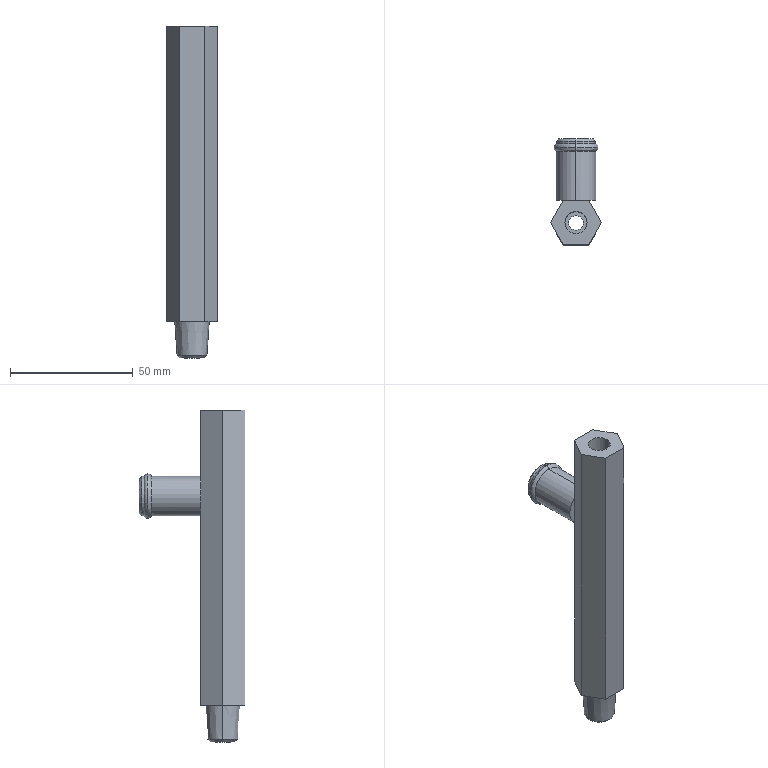Part | SolidWorks | features BaseBody 1 | 1 solid | 42 faces | box 20.785 x 43 x 135 mm | volume 30981 mm3 | plane 18 | cylinder 14 | cone 6 | spline 4 | commonest cylinder face diameters 9 x6 16 x4 6 x2 18 x2
STEP:
#1=CARTESIAN_POINT('',(0.,30.414,76.));
#2=VERTEX_POINT('',#1);
#3=CARTESIAN_POINT('',(0.,30.414,94.));
#4=VERTEX_POINT('',#3);
#5=CARTESIAN_POINT('',(0.,30.414,85.));
#6=DIRECTION('',(0.,-1.,0.));
#7=DIRECTION('',(0.,0.,-1.));
#8=AXIS2_PLACEMENT_3D('',#5,#6,#7);
#9=CIRCLE('',#8,9.);
#10=EDGE_CURVE('',#2,#4,#9,.T.);
#11=ORIENTED_EDGE('',*,*,#10,.T.);
#12=CARTESIAN_POINT('',(0.,29.,93.));
#13=VERTEX_POINT('',#12);
#14=CARTESIAN_POINT('',(0.,30.414,92.5));
#15=DIRECTION('',(1.,0.,0.));
#16=DIRECTION('',(0.,0.,1.));
#17=AXIS2_PLACEMENT_3D('',#14,#15,#16);
#18=CIRCLE('',#17,1.5);
#19=EDGE_CURVE('',#4,#13,#18,.T.);
#20=ORIENTED_EDGE('',*,*,#19,.T.);
#21=CARTESIAN_POINT('',(0.,29.,77.));
#22=VERTEX_POINT('',#21);
#23=CARTESIAN_POINT('',(0.,29.,85.));
#24=DIRECTION('',(0.,-1.,0.));
#25=DIRECTION('',(0.,0.,-1.));
#26=AXIS2_PLACEMENT_3D('',#23,#24,#25);
#27=CIRCLE('',#26,8.);
#28=EDGE_CURVE('',#22,#13,#27,.T.);
#29=ORIENTED_EDGE('',*,*,#28,.F.);
#30=CARTESIAN_POINT('',(0.,30.414,77.5));
#31=DIRECTION('',(-1.,0.,0.));
#32=DIRECTION('',(0.,0.,-1.));
#33=AXIS2_PLACEMENT_3D('',#30,#31,#32);
#34=CIRCLE('',#33,1.5);
#35=EDGE_CURVE('',#2,#22,#34,.T.);
#36=ORIENTED_EDGE('',*,*,#35,.F.);
#37=EDGE_LOOP('',(#11,#20,#29,#36));
#38=FACE_OUTER_BOUND('',#37,.T.);
#39=CARTESIAN_POINT('',(0.,30.414,94.));
#40=CARTESIAN_POINT('',(18.,30.414,94.));
#41=CARTESIAN_POINT('',(18.,30.414,76.));
#42=CARTESIAN_POINT('',(0.,30.414,76.));
#43=CARTESIAN_POINT('',(0.,29.756,94.));
#44=CARTESIAN_POINT('',(18.,29.756,94.));
#45=CARTESIAN_POINT('',(18.,29.756,76.));
#46=CARTESIAN_POINT('',(0.,29.756,76.));
#47=CARTESIAN_POINT('',(0.,29.219,93.62));
#48=CARTESIAN_POINT('',(17.24,29.219,93.62));
#49=CARTESIAN_POINT('',(17.24,29.219,76.38));
#50=CARTESIAN_POINT('',(0.,29.219,76.38));
#51=CARTESIAN_POINT('',(0.,29.,93.));
#52=CARTESIAN_POINT('',(16.,29.,93.));
#53=CARTESIAN_POINT('',(16.,29.,77.));
#54=CARTESIAN_POINT('',(0.,29.,77.));
#55=(BOUNDED_SURFACE()B_SPLINE_SURFACE(3,3,((#39,#40,#41,#42),(#43,#44,#45,#46),(#47,#48,#49,#50),(#51,#52,#53,#54)),.UNSPECIFIED.,.F.,.F.,.T.)B_SPLINE_SURFACE_WITH_KNOTS((4,4),(4,4),(0.,1.),(0.,1.),.UNSPECIFIED.)GEOMETRIC_REPRESENTATION_ITEM()RATIONAL_B_SPLINE_SURFACE(((1.,0.3333,0.3333,1.),(0.8777,0.2926,0.2926,0.8777),(0.8777,0.2926,0.2926,0.8777),(1.,0.3333,0.3333,1.)))REPRESENTATION_ITEM('')SURFACE());
#56=ADVANCED_FACE('',(#38),#55,.T.);
#57=CARTESIAN_POINT('',(0.,30.586,94.));
#58=VERTEX_POINT('',#57);
#59=CARTESIAN_POINT('',(0.,30.586,76.));
#60=VERTEX_POINT('',#59);
#61=CARTESIAN_POINT('',(0.,30.586,85.));
#62=DIRECTION('',(0.,-1.,0.));
#63=DIRECTION('',(0.,0.,1.));
#64=AXIS2_PLACEMENT_3D('',#61,#62,#63);
#65=CIRCLE('',#64,9.);
#66=EDGE_CURVE('',#58,#60,#65,.T.);
#67=ORIENTED_EDGE('',*,*,#66,.F.);
#68=CARTESIAN_POINT('',(0.,32.,93.));
#69=VERTEX_POINT('',#68);
#70=CARTESIAN_POINT('',(0.,30.586,92.5));
#71=DIRECTION('',(-1.,0.,0.));
#72=DIRECTION('',(0.,0.,1.));
#73=AXIS2_PLACEMENT_3D('',#70,#71,#72);
#74=CIRCLE('',#73,1.5);
#75=EDGE_CURVE('',#58,#69,#74,.T.);
#76=ORIENTED_EDGE('',*,*,#75,.T.);
#77=CARTESIAN_POINT('',(0.,32.,77.));
#78=VERTEX_POINT('',#77);
#79=CARTESIAN_POINT('',(0.,32.,85.));
#80=DIRECTION('',(0.,-1.,0.));
#81=DIRECTION('',(0.,0.,-1.));
#82=AXIS2_PLACEMENT_3D('',#79,#80,#81);
#83=CIRCLE('',#82,8.);
#84=EDGE_CURVE('',#69,#78,#83,.T.);
#85=ORIENTED_EDGE('',*,*,#84,.T.);
#86=CARTESIAN_POINT('',(0.,30.586,77.5));
#87=DIRECTION('',(1.,0.,0.));
#88=DIRECTION('',(0.,0.,-1.));
#89=AXIS2_PLACEMENT_3D('',#86,#87,#88);
#90=CIRCLE('',#89,1.5);
#91=EDGE_CURVE('',#60,#78,#90,.T.);
#92=ORIENTED_EDGE('',*,*,#91,.F.);
#93=EDGE_LOOP('',(#67,#76,#85,#92));
#94=FACE_OUTER_BOUND('',#93,.T.);
#95=CARTESIAN_POINT('',(0.,30.586,94.));
#96=CARTESIAN_POINT('',(-18.,30.586,94.));
#97=CARTESIAN_POINT('',(-18.,30.586,76.));
#98=CARTESIAN_POINT('',(0.,30.586,76.));
#99=CARTESIAN_POINT('',(0.,31.244,94.));
#100=CARTESIAN_POINT('',(-18.,31.244,94.));
#101=CARTESIAN_POINT('',(-18.,31.244,76.));
#102=CARTESIAN_POINT('',(0.,31.244,76.));
#103=CARTESIAN_POINT('',(0.,31.781,93.62));
#104=CARTESIAN_POINT('',(-17.24,31.781,93.62));
#105=CARTESIAN_POINT('',(-17.24,31.781,76.38));
#106=CARTESIAN_POINT('',(0.,31.781,76.38));
#107=CARTESIAN_POINT('',(0.,32.,93.));
#108=CARTESIAN_POINT('',(-16.,32.,93.));
#109=CARTESIAN_POINT('',(-16.,32.,77.));
#110=CARTESIAN_POINT('',(0.,32.,77.));
#111=(BOUNDED_SURFACE()B_SPLINE_SURFACE(3,3,((#95,#96,#97,#98),(#99,#100,#101,#102),(#103,#104,#105,#106),(#107,#108,#109,#110)),.UNSPECIFIED.,.F.,.F.,.F.)B_SPLINE_SURFACE_WITH_KNOTS((4,4),(4,4),(0.,1.),(0.,1.),.UNSPECIFIED.)GEOMETRIC_REPRESENTATION_ITEM()RATIONAL_B_SPLINE_SURFACE(((1.,0.3333,0.3333,1.),(0.8777,0.2926,0.2926,0.8777),(0.8777,0.2926,0.2926,0.8777),(1.,0.3333,0.3333,1.)))REPRESENTATION_ITEM('')SURFACE());
#112=ADVANCED_FACE('',(#94),#111,.T.);
#113=CARTESIAN_POINT('',(4.5,0.,120.));
#114=VERTEX_POINT('',#113);
#115=CARTESIAN_POINT('',(-4.5,0.,120.));
#116=VERTEX_POINT('',#115);
#117=CARTESIAN_POINT('',(0.,0.,120.));
#118=DIRECTION('',(0.,0.,-1.));
#119=DIRECTION('',(-1.,0.,0.));
#120=AXIS2_PLACEMENT_3D('',#117,#118,#119);
#121=CIRCLE('',#120,4.5);
#122=EDGE_CURVE('',#114,#116,#121,.T.);
#123=ORIENTED_EDGE('',*,*,#122,.F.);
#124=CARTESIAN_POINT('',(4.5,0.,0.));
#125=VERTEX_POINT('',#124);
#126=CARTESIAN_POINT('',(4.5,0.,120.));
#127=DIRECTION('',(0.,0.,-1.));
#128=VECTOR('',#127,1000.);
#129=LINE('',#126,#128);
#130=EDGE_CURVE('',#114,#125,#129,.T.);
#131=ORIENTED_EDGE('',*,*,#130,.T.);
#132=CARTESIAN_POINT('',(-4.5,0.,0.));
#133=VERTEX_POINT('',#132);
#134=CARTESIAN_POINT('',(0.,0.,0.));
#135=DIRECTION('',(0.,0.,1.));
#136=DIRECTION('',(-1.,0.,0.));
#137=AXIS2_PLACEMENT_3D('',#134,#135,#136);
#138=CIRCLE('',#137,4.5);
#139=EDGE_CURVE('',#133,#125,#138,.T.);
#140=ORIENTED_EDGE('',*,*,#139,.F.);
#141=CARTESIAN_POINT('',(-4.5,0.,120.));
#142=DIRECTION('',(0.,0.,-1.));
#143=VECTOR('',#142,1000.);
#144=LINE('',#141,#143);
#145=EDGE_CURVE('',#116,#133,#144,.T.);
#146=ORIENTED_EDGE('',*,*,#145,.F.);
#147=EDGE_LOOP('',(#123,#131,#140,#146));
#148=FACE_OUTER_BOUND('',#147,.T.);
#149=CARTESIAN_POINT('',(0.,0.,120.));
#150=DIRECTION('',(0.,0.,-1.));
#151=DIRECTION('',(-1.,0.,0.));
#152=AXIS2_PLACEMENT_3D('',#149,#150,#151);
#153=CYLINDRICAL_SURFACE('',#152,4.5);
#154=ADVANCED_FACE('',(#148),#153,.F.);
#155=CARTESIAN_POINT('',(-4.031,2.,83.));
#156=VERTEX_POINT('',#155);
#157=CARTESIAN_POINT('',(0.,4.5,80.5));
#158=VERTEX_POINT('',#157);
#159=CARTESIAN_POINT('',(-4.031,2.,83.));
#160=CARTESIAN_POINT('',(-3.25,3.574,81.426));
#161=CARTESIAN_POINT('',(-1.757,4.5,80.5));
#162=CARTESIAN_POINT('',(0.,4.5,80.5));
#163=(BOUNDED_CURVE()B_SPLINE_CURVE(3,(#159,#160,#161,#162),.UNSPECIFIED.,.F.,.T.)B_SPLINE_CURVE_WITH_KNOTS((4,4),(5.173,6.283),.UNSPECIFIED.)CURVE()GEOMETRIC_REPRESENTATION_ITEM()RATIONAL_B_SPLINE_CURVE((1.,0.8999,0.8999,1.))REPRESENTATION_ITEM(''));
#164=EDGE_CURVE('',#156,#158,#163,.T.);
#165=ORIENTED_EDGE('',*,*,#164,.T.);
#166=CARTESIAN_POINT('',(0.,29.,80.5));
#167=VERTEX_POINT('',#166);
#168=CARTESIAN_POINT('',(0.,2.,80.5));
#169=DIRECTION('',(0.,1.,0.));
#170=VECTOR('',#169,1000.);
#171=LINE('',#168,#170);
#172=EDGE_CURVE('',#158,#167,#171,.T.);
#173=ORIENTED_EDGE('',*,*,#172,.T.);
#174=CARTESIAN_POINT('',(0.,29.,89.5));
#175=VERTEX_POINT('',#174);
#176=CARTESIAN_POINT('',(0.,29.,85.));
#177=DIRECTION('',(0.,-1.,0.));
#178=DIRECTION('',(0.,0.,1.));
#179=AXIS2_PLACEMENT_3D('',#176,#177,#178);
#180=CIRCLE('',#179,4.5);
#181=EDGE_CURVE('',#175,#167,#180,.T.);
#182=ORIENTED_EDGE('',*,*,#181,.F.);
#183=CARTESIAN_POINT('',(0.,4.5,89.5));
#184=VERTEX_POINT('',#183);
#185=CARTESIAN_POINT('',(0.,2.,89.5));
#186=DIRECTION('',(0.,1.,0.));
#187=VECTOR('',#186,1000.);
#188=LINE('',#185,#187);
#189=EDGE_CURVE('',#184,#175,#188,.T.);
#190=ORIENTED_EDGE('',*,*,#189,.F.);
#191=CARTESIAN_POINT('',(-4.031,2.,87.));
#192=VERTEX_POINT('',#191);
#193=CARTESIAN_POINT('',(0.,4.5,89.5));
#194=CARTESIAN_POINT('',(-1.757,4.5,89.5));
#195=CARTESIAN_POINT('',(-3.25,3.574,88.574));
#196=CARTESIAN_POINT('',(-4.031,2.,87.));
#197=(BOUNDED_CURVE()B_SPLINE_CURVE(3,(#193,#194,#195,#196),.UNSPECIFIED.,.F.,.F.)B_SPLINE_CURVE_WITH_KNOTS((4,4),(0.,1.11),.UNSPECIFIED.)CURVE()GEOMETRIC_REPRESENTATION_ITEM()RATIONAL_B_SPLINE_CURVE((1.,0.8999,0.8999,1.))REPRESENTATION_ITEM(''));
#198=EDGE_CURVE('',#184,#192,#197,.T.);
#199=ORIENTED_EDGE('',*,*,#198,.T.);
#200=CARTESIAN_POINT('',(0.,2.,85.));
#201=DIRECTION('',(0.,1.,0.));
#202=DIRECTION('',(0.,0.,1.));
#203=AXIS2_PLACEMENT_3D('',#200,#201,#202);
#204=CIRCLE('',#203,4.5);
#205=EDGE_CURVE('',#156,#192,#204,.T.);
#206=ORIENTED_EDGE('',*,*,#205,.F.);
#207=EDGE_LOOP('',(#165,#173,#182,#190,#199,#206));
#208=FACE_OUTER_BOUND('',#207,.T.);
#209=CARTESIAN_POINT('',(0.,2.,85.));
#210=DIRECTION('',(0.,1.,0.));
#211=DIRECTION('',(0.,0.,1.));
#212=AXIS2_PLACEMENT_3D('',#209,#210,#211);
#213=CYLINDRICAL_SURFACE('',#212,4.5);
#214=ADVANCED_FACE('',(#208),#213,.F.);
#215=CARTESIAN_POINT('',(3.,0.,0.));
#216=VERTEX_POINT('',#215);
#217=CARTESIAN_POINT('',(-3.,0.,0.));
#218=VERTEX_POINT('',#217);
#219=CARTESIAN_POINT('',(0.,0.,0.));
#220=DIRECTION('',(0.,0.,-1.));
#221=DIRECTION('',(-1.,0.,0.));
#222=AXIS2_PLACEMENT_3D('',#219,#220,#221);
#223=CIRCLE('',#222,3.);
#224=EDGE_CURVE('',#216,#218,#223,.T.);
#225=ORIENTED_EDGE('',*,*,#224,.F.);
#226=CARTESIAN_POINT('',(3.,0.,-15.));
#227=VERTEX_POINT('',#226);
#228=CARTESIAN_POINT('',(3.,0.,0.));
#229=DIRECTION('',(0.,0.,-1.));
#230=VECTOR('',#229,1000.);
#231=LINE('',#228,#230);
#232=EDGE_CURVE('',#216,#227,#231,.T.);
#233=ORIENTED_EDGE('',*,*,#232,.T.);
#234=CARTESIAN_POINT('',(-3.,0.,-15.));
#235=VERTEX_POINT('',#234);
#236=CARTESIAN_POINT('',(0.,0.,-15.));
#237=DIRECTION('',(0.,0.,1.));
#238=DIRECTION('',(-1.,0.,0.));
#239=AXIS2_PLACEMENT_3D('',#236,#237,#238);
#240=CIRCLE('',#239,3.);
#241=EDGE_CURVE('',#235,#227,#240,.T.);
#242=ORIENTED_EDGE('',*,*,#241,.F.);
#243=CARTESIAN_POINT('',(-3.,0.,0.));
#244=DIRECTION('',(0.,0.,-1.));
#245=VECTOR('',#244,1000.);
#246=LINE('',#243,#245);
#247=EDGE_CURVE('',#218,#235,#246,.T.);
#248=ORIENTED_EDGE('',*,*,#247,.F.);
#249=EDGE_LOOP('',(#225,#233,#242,#248));
#250=FACE_OUTER_BOUND('',#249,.T.);
#251=CARTESIAN_POINT('',(0.,0.,0.));
#252=DIRECTION('',(0.,0.,-1.));
#253=DIRECTION('',(-1.,0.,0.));
#254=AXIS2_PLACEMENT_3D('',#251,#252,#253);
#255=CYLINDRICAL_SURFACE('',#254,3.);
#256=ADVANCED_FACE('',(#250),#255,.F.);
#257=ORIENTED_EDGE('',*,*,#28,.T.);
#258=CARTESIAN_POINT('',(0.,9.,93.));
#259=VERTEX_POINT('',#258);
#260=CARTESIAN_POINT('',(0.,29.,93.));
#261=DIRECTION('',(0.,-1.,0.));
#262=VECTOR('',#261,1000.);
#263=LINE('',#260,#262);
#264=EDGE_CURVE('',#13,#259,#263,.T.);
#265=ORIENTED_EDGE('',*,*,#264,.T.);
#266=CARTESIAN_POINT('',(5.196,9.,91.083));
#267=VERTEX_POINT('',#266);
#268=CARTESIAN_POINT('',(0.,9.,85.));
#269=DIRECTION('',(0.,-1.,0.));
#270=DIRECTION('',(0.,0.,-1.));
#271=AXIS2_PLACEMENT_3D('',#268,#269,#270);
#272=CIRCLE('',#271,8.);
#273=EDGE_CURVE('',#267,#259,#272,.T.);
#274=ORIENTED_EDGE('',*,*,#273,.F.);
#275=CARTESIAN_POINT('',(5.196,9.,78.917));
#276=VERTEX_POINT('',#275);
#277=CARTESIAN_POINT('',(0.,9.,85.));
#278=DIRECTION('',(0.,1.,0.));
#279=DIRECTION('',(0.,0.,-1.));
#280=AXIS2_PLACEMENT_3D('',#277,#278,#279);
#281=CIRCLE('',#280,8.);
#282=EDGE_CURVE('',#267,#276,#281,.T.);
#283=ORIENTED_EDGE('',*,*,#282,.T.);
#284=CARTESIAN_POINT('',(0.,9.,77.));
#285=VERTEX_POINT('',#284);
#286=CARTESIAN_POINT('',(0.,9.,85.));
#287=DIRECTION('',(0.,-1.,0.));
#288=DIRECTION('',(0.,0.,-1.));
#289=AXIS2_PLACEMENT_3D('',#286,#287,#288);
#290=CIRCLE('',#289,8.);
#291=EDGE_CURVE('',#285,#276,#290,.T.);
#292=ORIENTED_EDGE('',*,*,#291,.F.);
#293=CARTESIAN_POINT('',(0.,29.,77.));
#294=DIRECTION('',(0.,-1.,0.));
#295=VECTOR('',#294,1000.);
#296=LINE('',#293,#295);
#297=EDGE_CURVE('',#22,#285,#296,.T.);
#298=ORIENTED_EDGE('',*,*,#297,.F.);
#299=EDGE_LOOP('',(#257,#265,#274,#283,#292,#298));
#300=FACE_OUTER_BOUND('',#299,.T.);
#301=CARTESIAN_POINT('',(0.,29.,85.));
#302=DIRECTION('',(0.,-1.,0.));
#303=DIRECTION('',(0.,0.,-1.));
#304=AXIS2_PLACEMENT_3D('',#301,#302,#303);
#305=CYLINDRICAL_SURFACE('',#304,8.);
#306=ADVANCED_FACE('',(#300),#305,.T.);
#307=CARTESIAN_POINT('',(6.071,0.,-13.929));
#308=VERTEX_POINT('',#307);
#309=CARTESIAN_POINT('',(-6.071,0.,-13.929));
#310=VERTEX_POINT('',#309);
#311=CARTESIAN_POINT('',(0.,0.,-13.929));
#312=DIRECTION('',(0.,0.,1.));
#313=DIRECTION('',(1.,0.,0.));
#314=AXIS2_PLACEMENT_3D('',#311,#312,#313);
#315=CIRCLE('',#314,6.071);
#316=EDGE_CURVE('',#308,#310,#315,.T.);
#317=ORIENTED_EDGE('',*,*,#316,.T.);
#318=CARTESIAN_POINT('',(-7.,0.,0.));
#319=VERTEX_POINT('',#318);
#320=CARTESIAN_POINT('',(-7.,0.,0.));
#321=DIRECTION('',(-0.06652,0.,0.9978));
#322=VECTOR('',#321,1000.);
#323=LINE('',#320,#322);
#324=EDGE_CURVE('',#310,#319,#323,.T.);
#325=ORIENTED_EDGE('',*,*,#324,.T.);
#326=CARTESIAN_POINT('',(7.,0.,0.));
#327=VERTEX_POINT('',#326);
#328=CARTESIAN_POINT('',(0.,0.,0.));
#329=DIRECTION('',(0.,0.,-1.));
#330=DIRECTION('',(1.,0.,0.));
#331=AXIS2_PLACEMENT_3D('',#328,#329,#330);
#332=CIRCLE('',#331,7.);
#333=EDGE_CURVE('',#319,#327,#332,.T.);
#334=ORIENTED_EDGE('',*,*,#333,.T.);
#335=CARTESIAN_POINT('',(7.,0.,0.));
#336=DIRECTION('',(0.06652,0.,0.9978));
#337=VECTOR('',#336,1000.);
#338=LINE('',#335,#337);
#339=EDGE_CURVE('',#308,#327,#338,.T.);
#340=ORIENTED_EDGE('',*,*,#339,.F.);
#341=EDGE_LOOP('',(#317,#325,#334,#340));
#342=FACE_OUTER_BOUND('',#341,.T.);
#343=CARTESIAN_POINT('',(0.,0.,0.));
#344=DIRECTION('',(0.,0.,1.));
#345=DIRECTION('',(1.,0.,0.));
#346=AXIS2_PLACEMENT_3D('',#343,#344,#345);
#347=CONICAL_SURFACE('',#346,7.,0.06657);
#348=ADVANCED_FACE('',(#342),#347,.T.);
#349=CARTESIAN_POINT('',(5.,0.,-15.));
#350=VERTEX_POINT('',#349);
#351=CARTESIAN_POINT('',(-5.,0.,-15.));
#352=VERTEX_POINT('',#351);
#353=CARTESIAN_POINT('',(0.,0.,-15.));
#354=DIRECTION('',(0.,0.,1.));
#355=DIRECTION('',(1.,0.,0.));
#356=AXIS2_PLACEMENT_3D('',#353,#354,#355);
#357=CIRCLE('',#356,5.);
#358=EDGE_CURVE('',#350,#352,#357,.T.);
#359=ORIENTED_EDGE('',*,*,#358,.T.);
#360=CARTESIAN_POINT('',(-6.071,0.,-13.929));
#361=DIRECTION('',(-0.7071,0.,0.7071));
#362=VECTOR('',#361,1000.);
#363=LINE('',#360,#362);
#364=EDGE_CURVE('',#352,#310,#363,.T.);
#365=ORIENTED_EDGE('',*,*,#364,.T.);
#366=ORIENTED_EDGE('',*,*,#316,.F.);
#367=CARTESIAN_POINT('',(6.071,0.,-13.929));
#368=DIRECTION('',(0.7071,0.,0.7071));
#369=VECTOR('',#368,1000.);
#370=LINE('',#367,#369);
#371=EDGE_CURVE('',#350,#308,#370,.T.);
#372=ORIENTED_EDGE('',*,*,#371,.F.);
#373=EDGE_LOOP('',(#359,#365,#366,#372));
#374=FACE_OUTER_BOUND('',#373,.T.);
#375=CARTESIAN_POINT('',(0.,0.,-13.929));
#376=DIRECTION('',(0.,0.,1.));
#377=DIRECTION('',(1.,0.,0.));
#378=AXIS2_PLACEMENT_3D('',#375,#376,#377);
#379=CONICAL_SURFACE('',#378,6.071,0.7854);
#380=ADVANCED_FACE('',(#374),#379,.T.);
#381=ORIENTED_EDGE('',*,*,#10,.F.);
#382=CARTESIAN_POINT('',(0.,30.414,76.));
#383=DIRECTION('',(0.,1.,0.));
#384=VECTOR('',#383,1000.);
#385=LINE('',#382,#384);
#386=EDGE_CURVE('',#2,#60,#385,.T.);
#387=ORIENTED_EDGE('',*,*,#386,.T.);
#388=CARTESIAN_POINT('',(0.,30.586,85.));
#389=DIRECTION('',(0.,-1.,0.));
#390=DIRECTION('',(0.,0.,1.));
#391=AXIS2_PLACEMENT_3D('',#388,#389,#390);
#392=CIRCLE('',#391,9.);
#393=EDGE_CURVE('',#60,#58,#392,.T.);
#394=ORIENTED_EDGE('',*,*,#393,.T.);
#395=CARTESIAN_POINT('',(0.,30.414,94.));
#396=DIRECTION('',(0.,1.,0.));
#397=VECTOR('',#396,1000.);
#398=LINE('',#395,#397);
#399=EDGE_CURVE('',#4,#58,#398,.T.);
#400=ORIENTED_EDGE('',*,*,#399,.F.);
#401=EDGE_LOOP('',(#381,#387,#394,#400));
#402=FACE_OUTER_BOUND('',#401,.T.);
#403=CARTESIAN_POINT('',(0.,30.414,85.));
#404=DIRECTION('',(0.,1.,0.));
#405=DIRECTION('',(0.,0.,1.));
#406=AXIS2_PLACEMENT_3D('',#403,#404,#405);
#407=CYLINDRICAL_SURFACE('',#406,9.);
#408=ADVANCED_FACE('',(#402),#407,.T.);
#409=CARTESIAN_POINT('',(0.,33.,77.));
#410=VERTEX_POINT('',#409);
#411=CARTESIAN_POINT('',(0.,33.,93.));
#412=VERTEX_POINT('',#411);
#413=CARTESIAN_POINT('',(0.,33.,85.));
#414=DIRECTION('',(0.,-1.,0.));
#415=DIRECTION('',(0.,0.,-1.));
#416=AXIS2_PLACEMENT_3D('',#413,#414,#415);
#417=CIRCLE('',#416,8.);
#418=EDGE_CURVE('',#410,#412,#417,.T.);
#419=ORIENTED_EDGE('',*,*,#418,.T.);
#420=CARTESIAN_POINT('',(0.,33.,93.));
#421=DIRECTION('',(0.,-1.,0.));
#422=VECTOR('',#421,1000.);
#423=LINE('',#420,#422);
#424=EDGE_CURVE('',#412,#69,#423,.T.);
#425=ORIENTED_EDGE('',*,*,#424,.T.);
#426=CARTESIAN_POINT('',(0.,32.,85.));
#427=DIRECTION('',(0.,-1.,0.));
#428=DIRECTION('',(0.,0.,-1.));
#429=AXIS2_PLACEMENT_3D('',#426,#427,#428);
#430=CIRCLE('',#429,8.);
#431=EDGE_CURVE('',#78,#69,#430,.T.);
#432=ORIENTED_EDGE('',*,*,#431,.F.);
#433=CARTESIAN_POINT('',(0.,33.,77.));
#434=DIRECTION('',(0.,-1.,0.));
#435=VECTOR('',#434,1000.);
#436=LINE('',#433,#435);
#437=EDGE_CURVE('',#410,#78,#436,.T.);
#438=ORIENTED_EDGE('',*,*,#437,.F.);
#439=EDGE_LOOP('',(#419,#425,#432,#438));
#440=FACE_OUTER_BOUND('',#439,.T.);
#441=CARTESIAN_POINT('',(0.,33.,85.));
#442=DIRECTION('',(0.,-1.,0.));
#443=DIRECTION('',(0.,0.,-1.));
#444=AXIS2_PLACEMENT_3D('',#441,#442,#443);
#445=CYLINDRICAL_SURFACE('',#444,8.);
#446=ADVANCED_FACE('',(#440),#445,.T.);
#447=CARTESIAN_POINT('',(0.,34.,78.));
#448=VERTEX_POINT('',#447);
#449=CARTESIAN_POINT('',(0.,34.,92.));
#450=VERTEX_POINT('',#449);
#451=CARTESIAN_POINT('',(0.,34.,85.));
#452=DIRECTION('',(0.,-1.,0.));
#453=DIRECTION('',(0.,0.,-1.));
#454=AXIS2_PLACEMENT_3D('',#451,#452,#453);
#455=CIRCLE('',#454,7.);
#456=EDGE_CURVE('',#448,#450,#455,.T.);
#457=ORIENTED_EDGE('',*,*,#456,.T.);
#458=CARTESIAN_POINT('',(0.,33.,93.));
#459=DIRECTION('',(0.,-0.7071,0.7071));
#460=VECTOR('',#459,1000.);
#461=LINE('',#458,#460);
#462=EDGE_CURVE('',#450,#412,#461,.T.);
#463=ORIENTED_EDGE('',*,*,#462,.T.);
#464=ORIENTED_EDGE('',*,*,#418,.F.);
#465=CARTESIAN_POINT('',(0.,33.,77.));
#466=DIRECTION('',(0.,-0.7071,-0.7071));
#467=VECTOR('',#466,1000.);
#468=LINE('',#465,#467);
#469=EDGE_CURVE('',#448,#410,#468,.T.);
#470=ORIENTED_EDGE('',*,*,#469,.F.);
#471=EDGE_LOOP('',(#457,#463,#464,#470));
#472=FACE_OUTER_BOUND('',#471,.T.);
#473=CARTESIAN_POINT('',(0.,33.,85.));
#474=DIRECTION('',(0.,-1.,0.));
#475=DIRECTION('',(0.,0.,-1.));
#476=AXIS2_PLACEMENT_3D('',#473,#474,#475);
#477=CONICAL_SURFACE('',#476,8.,0.7854);
#478=ADVANCED_FACE('',(#472),#477,.T.);
#479=CARTESIAN_POINT('',(0.,34.,89.5));
#480=VERTEX_POINT('',#479);
#481=CARTESIAN_POINT('',(0.,34.,80.5));
#482=VERTEX_POINT('',#481);
#483=CARTESIAN_POINT('',(0.,34.,85.));
#484=DIRECTION('',(0.,-1.,0.));
#485=DIRECTION('',(0.,0.,-1.));
#486=AXIS2_PLACEMENT_3D('',#483,#484,#485);
#487=CIRCLE('',#486,4.5);
#488=EDGE_CURVE('',#480,#482,#487,.T.);
#489=ORIENTED_EDGE('',*,*,#488,.F.);
#490=CARTESIAN_POINT('',(0.,32.,89.5));
#491=VERTEX_POINT('',#490);
#492=CARTESIAN_POINT('',(0.,34.,89.5));
#493=DIRECTION('',(0.,-1.,0.));
#494=VECTOR('',#493,1000.);
#495=LINE('',#492,#494);
#496=EDGE_CURVE('',#480,#491,#495,.T.);
#497=ORIENTED_EDGE('',*,*,#496,.T.);
#498=CARTESIAN_POINT('',(0.,32.,80.5));
#499=VERTEX_POINT('',#498);
#500=CARTESIAN_POINT('',(0.,32.,85.));
#501=DIRECTION('',(0.,1.,0.));
#502=DIRECTION('',(0.,0.,-1.));
#503=AXIS2_PLACEMENT_3D('',#500,#501,#502);
#504=CIRCLE('',#503,4.5);
#505=EDGE_CURVE('',#499,#491,#504,.T.);
#506=ORIENTED_EDGE('',*,*,#505,.F.);
#507=CARTESIAN_POINT('',(0.,34.,80.5));
#508=DIRECTION('',(0.,-1.,0.));
#509=VECTOR('',#508,1000.);
#510=LINE('',#507,#509);
#511=EDGE_CURVE('',#482,#499,#510,.T.);
#512=ORIENTED_EDGE('',*,*,#511,.F.);
#513=EDGE_LOOP('',(#489,#497,#506,#512));
#514=FACE_OUTER_BOUND('',#513,.T.);
#515=CARTESIAN_POINT('',(0.,34.,85.));
#516=DIRECTION('',(0.,-1.,0.));
#517=DIRECTION('',(0.,0.,-1.));
#518=AXIS2_PLACEMENT_3D('',#515,#516,#517);
#519=CYLINDRICAL_SURFACE('',#518,4.5);
#520=ADVANCED_FACE('',(#514),#519,.F.);
#521=ORIENTED_EDGE('',*,*,#130,.F.);
#522=CARTESIAN_POINT('',(0.,0.,120.));
#523=DIRECTION('',(0.,0.,-1.));
#524=DIRECTION('',(-1.,0.,0.));
#525=AXIS2_PLACEMENT_3D('',#522,#523,#524);
#526=CIRCLE('',#525,4.5);
#527=EDGE_CURVE('',#116,#114,#526,.T.);
#528=ORIENTED_EDGE('',*,*,#527,.F.);
#529=ORIENTED_EDGE('',*,*,#145,.T.);
#530=CARTESIAN_POINT('',(0.,0.,0.));
#531=DIRECTION('',(0.,0.,1.));
#532=DIRECTION('',(-1.,0.,0.));
#533=AXIS2_PLACEMENT_3D('',#530,#531,#532);
#534=CIRCLE('',#533,4.5);
#535=EDGE_CURVE('',#125,#133,#534,.T.);
#536=ORIENTED_EDGE('',*,*,#535,.F.);
#537=EDGE_LOOP('',(#521,#528,#529,#536));
#538=FACE_OUTER_BOUND('',#537,.T.);
#539=CARTESIAN_POINT('',(4.031,2.,87.));
#540=VERTEX_POINT('',#539);
#541=CARTESIAN_POINT('',(4.031,2.,87.));
#542=CARTESIAN_POINT('',(3.25,3.574,88.574));
#543=CARTESIAN_POINT('',(1.757,4.5,89.5));
#544=CARTESIAN_POINT('',(0.,4.5,89.5));
#545=(BOUNDED_CURVE()B_SPLINE_CURVE(3,(#541,#542,#543,#544),.UNSPECIFIED.,.F.,.T.)B_SPLINE_CURVE_WITH_KNOTS((4,4),(5.173,6.283),.UNSPECIFIED.)CURVE()GEOMETRIC_REPRESENTATION_ITEM()RATIONAL_B_SPLINE_CURVE((1.,0.8999,0.8999,1.))REPRESENTATION_ITEM(''));
#546=EDGE_CURVE('',#540,#184,#545,.T.);
#547=ORIENTED_EDGE('',*,*,#546,.F.);
#548=CARTESIAN_POINT('',(4.031,2.,83.));
#549=VERTEX_POINT('',#548);
#550=CARTESIAN_POINT('',(4.031,2.,120.));
#551=DIRECTION('',(0.,0.,1.));
#552=VECTOR('',#551,1000.);
#553=LINE('',#550,#552);
#554=EDGE_CURVE('',#549,#540,#553,.T.);
#555=ORIENTED_EDGE('',*,*,#554,.F.);
#556=CARTESIAN_POINT('',(0.,4.5,80.5));
#557=CARTESIAN_POINT('',(1.757,4.5,80.5));
#558=CARTESIAN_POINT('',(3.25,3.574,81.426));
#559=CARTESIAN_POINT('',(4.031,2.,83.));
#560=(BOUNDED_CURVE()B_SPLINE_CURVE(3,(#556,#557,#558,#559),.UNSPECIFIED.,.F.,.F.)B_SPLINE_CURVE_WITH_KNOTS((4,4),(0.,1.11),.UNSPECIFIED.)CURVE()GEOMETRIC_REPRESENTATION_ITEM()RATIONAL_B_SPLINE_CURVE((1.,0.8999,0.8999,1.))REPRESENTATION_ITEM(''));
#561=EDGE_CURVE('',#158,#549,#560,.T.);
#562=ORIENTED_EDGE('',*,*,#561,.F.);
#563=ORIENTED_EDGE('',*,*,#164,.F.);
#564=CARTESIAN_POINT('',(-4.031,2.,120.));
#565=DIRECTION('',(0.,0.,-1.));
#566=VECTOR('',#565,1000.);
#567=LINE('',#564,#566);
#568=EDGE_CURVE('',#192,#156,#567,.T.);
#569=ORIENTED_EDGE('',*,*,#568,.F.);
#570=ORIENTED_EDGE('',*,*,#198,.F.);
#571=EDGE_LOOP('',(#547,#555,#562,#563,#569,#570));
#572=FACE_BOUND('',#571,.T.);
#573=CARTESIAN_POINT('',(0.,0.,120.));
#574=DIRECTION('',(0.,0.,-1.));
#575=DIRECTION('',(-1.,0.,0.));
#576=AXIS2_PLACEMENT_3D('',#573,#574,#575);
#577=CYLINDRICAL_SURFACE('',#576,4.5);
#578=ADVANCED_FACE('',(#538,#572),#577,.F.);
#579=ORIENTED_EDGE('',*,*,#527,.T.);
#580=ORIENTED_EDGE('',*,*,#122,.T.);
#581=EDGE_LOOP('',(#579,#580));
#582=FACE_BOUND('',#581,.T.);
#583=CARTESIAN_POINT('',(-5.196,9.,120.));
#584=VERTEX_POINT('',#583);
#585=CARTESIAN_POINT('',(-10.392,0.000000001,120.));
#586=VERTEX_POINT('',#585);
#587=CARTESIAN_POINT('',(-5.196,9.,120.));
#588=DIRECTION('',(-0.5,-0.866,0.));
#589=VECTOR('',#588,1000.);
#590=LINE('',#587,#589);
#591=EDGE_CURVE('',#584,#586,#590,.T.);
#592=ORIENTED_EDGE('',*,*,#591,.T.);
#593=CARTESIAN_POINT('',(-5.196,-9.,120.));
#594=VERTEX_POINT('',#593);
#595=CARTESIAN_POINT('',(-10.392,0.,120.));
#596=DIRECTION('',(0.5,-0.866,0.));
#597=VECTOR('',#596,1000.);
#598=LINE('',#595,#597);
#599=EDGE_CURVE('',#586,#594,#598,.T.);
#600=ORIENTED_EDGE('',*,*,#599,.T.);
#601=CARTESIAN_POINT('',(5.196,-9.,120.));
#602=VERTEX_POINT('',#601);
#603=CARTESIAN_POINT('',(0.000000004,-9.,120.));
#604=DIRECTION('',(1.,0.,0.));
#605=VECTOR('',#604,1000.);
#606=LINE('',#603,#605);
#607=EDGE_CURVE('',#594,#602,#606,.T.);
#608=ORIENTED_EDGE('',*,*,#607,.T.);
#609=CARTESIAN_POINT('',(10.392,0.000000003,120.));
#610=VERTEX_POINT('',#609);
#611=CARTESIAN_POINT('',(5.196,-9.,120.));
#612=DIRECTION('',(0.5,0.866,0.));
#613=VECTOR('',#612,1000.);
#614=LINE('',#611,#613);
#615=EDGE_CURVE('',#602,#610,#614,.T.);
#616=ORIENTED_EDGE('',*,*,#615,.T.);
#617=CARTESIAN_POINT('',(5.196,9.,120.));
#618=VERTEX_POINT('',#617);
#619=CARTESIAN_POINT('',(10.392,0.000000005,120.));
#620=DIRECTION('',(-0.5,0.866,0.));
#621=VECTOR('',#620,1000.);
#622=LINE('',#619,#621);
#623=EDGE_CURVE('',#610,#618,#622,.T.);
#624=ORIENTED_EDGE('',*,*,#623,.T.);
#625=CARTESIAN_POINT('',(0.000000004,9.,120.));
#626=DIRECTION('',(-1.,0.,0.));
#627=VECTOR('',#626,1000.);
#628=LINE('',#625,#627);
#629=EDGE_CURVE('',#618,#584,#628,.T.);
#630=ORIENTED_EDGE('',*,*,#629,.T.);
#631=EDGE_LOOP('',(#592,#600,#608,#616,#624,#630));
#632=FACE_OUTER_BOUND('',#631,.T.);
#633=CARTESIAN_POINT('',(0.000000004,0.,120.));
#634=DIRECTION('',(0.,0.,1.));
#635=DIRECTION('',(1.,0.,0.));
#636=AXIS2_PLACEMENT_3D('',#633,#634,#635);
#637=PLANE('',#636);
#638=ADVANCED_FACE('',(#582,#632),#637,.T.);
#639=CARTESIAN_POINT('',(0.,0.,0.));
#640=DIRECTION('',(0.,0.,-1.));
#641=DIRECTION('',(-1.,0.,0.));
#642=AXIS2_PLACEMENT_3D('',#639,#640,#641);
#643=CIRCLE('',#642,3.);
#644=EDGE_CURVE('',#218,#216,#643,.T.);
#645=ORIENTED_EDGE('',*,*,#644,.T.);
#646=ORIENTED_EDGE('',*,*,#224,.T.);
#647=EDGE_LOOP('',(#645,#646));
#648=FACE_BOUND('',#647,.T.);
#649=ORIENTED_EDGE('',*,*,#139,.T.);
#650=ORIENTED_EDGE('',*,*,#535,.T.);
#651=EDGE_LOOP('',(#649,#650));
#652=FACE_OUTER_BOUND('',#651,.T.);
#653=CARTESIAN_POINT('',(0.,0.,0.));
#654=DIRECTION('',(0.,0.,1.));
#655=DIRECTION('',(1.,0.,0.));
#656=AXIS2_PLACEMENT_3D('',#653,#654,#655);
#657=PLANE('',#656);
#658=ADVANCED_FACE('',(#648,#652),#657,.T.);
#659=ORIENTED_EDGE('',*,*,#172,.F.);
#660=ORIENTED_EDGE('',*,*,#561,.T.);
#661=CARTESIAN_POINT('',(0.,2.,85.));
#662=DIRECTION('',(0.,1.,0.));
#663=DIRECTION('',(0.,0.,1.));
#664=AXIS2_PLACEMENT_3D('',#661,#662,#663);
#665=CIRCLE('',#664,4.5);
#666=EDGE_CURVE('',#540,#549,#665,.T.);
#667=ORIENTED_EDGE('',*,*,#666,.F.);
#668=ORIENTED_EDGE('',*,*,#546,.T.);
#669=ORIENTED_EDGE('',*,*,#189,.T.);
#670=CARTESIAN_POINT('',(0.,29.,85.));
#671=DIRECTION('',(0.,-1.,0.));
#672=DIRECTION('',(0.,0.,1.));
#673=AXIS2_PLACEMENT_3D('',#670,#671,#672);
#674=CIRCLE('',#673,4.5);
#675=EDGE_CURVE('',#167,#175,#674,.T.);
#676=ORIENTED_EDGE('',*,*,#675,.F.);
#677=EDGE_LOOP('',(#659,#660,#667,#668,#669,#676));
#678=FACE_OUTER_BOUND('',#677,.T.);
#679=CARTESIAN_POINT('',(0.,2.,85.));
#680=DIRECTION('',(0.,1.,0.));
#681=DIRECTION('',(0.,0.,1.));
#682=AXIS2_PLACEMENT_3D('',#679,#680,#681);
#683=CYLINDRICAL_SURFACE('',#682,4.5);
#684=ADVANCED_FACE('',(#678),#683,.F.);
#685=ORIENTED_EDGE('',*,*,#568,.T.);
#686=ORIENTED_EDGE('',*,*,#205,.T.);
#687=EDGE_LOOP('',(#685,#686));
#688=FACE_OUTER_BOUND('',#687,.T.);
#689=CARTESIAN_POINT('',(-4.266,2.,85.));
#690=DIRECTION('',(0.,1.,0.));
#691=DIRECTION('',(0.,0.,1.));
#692=AXIS2_PLACEMENT_3D('',#689,#690,#691);
#693=PLANE('',#692);
#694=ADVANCED_FACE('',(#688),#693,.T.);
#695=ORIENTED_EDGE('',*,*,#599,.F.);
#696=CARTESIAN_POINT('',(-10.392,0.000000001,0.));
#697=VERTEX_POINT('',#696);
#698=CARTESIAN_POINT('',(-10.392,0.,60.));
#699=DIRECTION('',(0.,0.,1.));
#700=VECTOR('',#699,1000.);
#701=LINE('',#698,#700);
#702=EDGE_CURVE('',#697,#586,#701,.T.);
#703=ORIENTED_EDGE('',*,*,#702,.F.);
#704=CARTESIAN_POINT('',(-5.196,-9.,0.));
#705=VERTEX_POINT('',#704);
#706=CARTESIAN_POINT('',(-7.794,-4.5,0.));
#707=DIRECTION('',(-0.5,0.866,0.));
#708=VECTOR('',#707,1000.);
#709=LINE('',#706,#708);
#710=EDGE_CURVE('',#705,#697,#709,.T.);
#711=ORIENTED_EDGE('',*,*,#710,.F.);
#712=CARTESIAN_POINT('',(-5.196,-9.,60.));
#713=DIRECTION('',(0.,0.,-1.));
#714=VECTOR('',#713,1000.);
#715=LINE('',#712,#714);
#716=EDGE_CURVE('',#594,#705,#715,.T.);
#717=ORIENTED_EDGE('',*,*,#716,.F.);
#718=EDGE_LOOP('',(#695,#703,#711,#717));
#719=FACE_OUTER_BOUND('',#718,.T.);
#720=CARTESIAN_POINT('',(-7.794,-4.5,60.));
#721=DIRECTION('',(0.866,0.5,0.));
#722=DIRECTION('',(-0.5,0.866,0.));
#723=AXIS2_PLACEMENT_3D('',#720,#721,#722);
#724=PLANE('',#723);
#725=ADVANCED_FACE('',(#719),#724,.F.);
#726=CARTESIAN_POINT('',(-5.196,9.,0.));
#727=VERTEX_POINT('',#726);
#728=CARTESIAN_POINT('',(-7.794,4.5,0.));
#729=DIRECTION('',(0.5,0.866,0.));
#730=VECTOR('',#729,1000.);
#731=LINE('',#728,#730);
#732=EDGE_CURVE('',#697,#727,#731,.T.);
#733=ORIENTED_EDGE('',*,*,#732,.F.);
#734=ORIENTED_EDGE('',*,*,#702,.T.);
#735=ORIENTED_EDGE('',*,*,#591,.F.);
#736=CARTESIAN_POINT('',(-5.196,9.,91.083));
#737=VERTEX_POINT('',#736);
#738=CARTESIAN_POINT('',(-5.196,9.,60.));
#739=DIRECTION('',(0.,0.,1.));
#740=VECTOR('',#739,1000.);
#741=LINE('',#738,#740);
#742=EDGE_CURVE('',#737,#584,#741,.T.);
#743=ORIENTED_EDGE('',*,*,#742,.F.);
#744=CARTESIAN_POINT('',(-5.196,9.,78.917));
#745=VERTEX_POINT('',#744);
#746=CARTESIAN_POINT('',(-5.196,9.,60.));
#747=DIRECTION('',(0.,0.,1.));
#748=VECTOR('',#747,1000.);
#749=LINE('',#746,#748);
#750=EDGE_CURVE('',#745,#737,#749,.T.);
#751=ORIENTED_EDGE('',*,*,#750,.F.);
#752=CARTESIAN_POINT('',(-5.196,9.,60.));
#753=DIRECTION('',(0.,0.,1.));
#754=VECTOR('',#753,1000.);
#755=LINE('',#752,#754);
#756=EDGE_CURVE('',#727,#745,#755,.T.);
#757=ORIENTED_EDGE('',*,*,#756,.F.);
#758=EDGE_LOOP('',(#733,#734,#735,#743,#751,#757));
#759=FACE_OUTER_BOUND('',#758,.T.);
#760=CARTESIAN_POINT('',(-7.794,4.5,60.));
#761=DIRECTION('',(0.866,-0.5,0.));
#762=DIRECTION('',(0.5,0.866,0.));
#763=AXIS2_PLACEMENT_3D('',#760,#761,#762);
#764=PLANE('',#763);
#765=ADVANCED_FACE('',(#759),#764,.F.);
#766=CARTESIAN_POINT('',(5.196,9.,60.));
#767=DIRECTION('',(0.,0.,-1.));
#768=VECTOR('',#767,1000.);
#769=LINE('',#766,#768);
#770=EDGE_CURVE('',#618,#267,#769,.T.);
#771=ORIENTED_EDGE('',*,*,#770,.T.);
#772=ORIENTED_EDGE('',*,*,#273,.T.);
#773=CARTESIAN_POINT('',(0.,9.,85.));
#774=DIRECTION('',(0.,-1.,0.));
#775=DIRECTION('',(0.,0.,-1.));
#776=AXIS2_PLACEMENT_3D('',#773,#774,#775);
#777=CIRCLE('',#776,8.);
#778=EDGE_CURVE('',#259,#737,#777,.T.);
#779=ORIENTED_EDGE('',*,*,#778,.T.);
#780=ORIENTED_EDGE('',*,*,#742,.T.);
#781=ORIENTED_EDGE('',*,*,#629,.F.);
#782=EDGE_LOOP('',(#771,#772,#779,#780,#781));
#783=FACE_OUTER_BOUND('',#782,.T.);
#784=CARTESIAN_POINT('',(0.,9.,60.));
#785=DIRECTION('',(0.,1.,0.));
#786=DIRECTION('',(0.,0.,1.));
#787=AXIS2_PLACEMENT_3D('',#784,#785,#786);
#788=PLANE('',#787);
#789=ADVANCED_FACE('',(#783),#788,.T.);
#790=CARTESIAN_POINT('',(5.196,9.,0.));
#791=VERTEX_POINT('',#790);
#792=CARTESIAN_POINT('',(5.196,9.,60.));
#793=DIRECTION('',(0.,0.,1.));
#794=VECTOR('',#793,1000.);
#795=LINE('',#792,#794);
#796=EDGE_CURVE('',#791,#276,#795,.T.);
#797=ORIENTED_EDGE('',*,*,#796,.T.);
#798=CARTESIAN_POINT('',(5.196,9.,60.));
#799=DIRECTION('',(0.,0.,1.));
#800=VECTOR('',#799,1000.);
#801=LINE('',#798,#800);
#802=EDGE_CURVE('',#276,#267,#801,.T.);
#803=ORIENTED_EDGE('',*,*,#802,.T.);
#804=ORIENTED_EDGE('',*,*,#770,.F.);
#805=ORIENTED_EDGE('',*,*,#623,.F.);
#806=CARTESIAN_POINT('',(10.392,0.000000002,0.));
#807=VERTEX_POINT('',#806);
#808=CARTESIAN_POINT('',(10.392,0.000000004,60.));
#809=DIRECTION('',(0.,0.,-1.));
#810=VECTOR('',#809,1000.);
#811=LINE('',#808,#810);
#812=EDGE_CURVE('',#610,#807,#811,.T.);
#813=ORIENTED_EDGE('',*,*,#812,.T.);
#814=CARTESIAN_POINT('',(7.794,4.5,0.));
#815=DIRECTION('',(-0.5,0.866,0.));
#816=VECTOR('',#815,1000.);
#817=LINE('',#814,#816);
#818=EDGE_CURVE('',#807,#791,#817,.T.);
#819=ORIENTED_EDGE('',*,*,#818,.T.);
#820=EDGE_LOOP('',(#797,#803,#804,#805,#813,#819));
#821=FACE_OUTER_BOUND('',#820,.T.);
#822=CARTESIAN_POINT('',(7.794,4.5,60.));
#823=DIRECTION('',(0.866,0.5,0.));
#824=DIRECTION('',(-0.5,0.866,0.));
#825=AXIS2_PLACEMENT_3D('',#822,#823,#824);
#826=PLANE('',#825);
#827=ADVANCED_FACE('',(#821),#826,.T.);
#828=CARTESIAN_POINT('',(5.196,-9.,0.));
#829=VERTEX_POINT('',#828);
#830=CARTESIAN_POINT('',(5.196,-9.,60.));
#831=DIRECTION('',(0.,0.,-1.));
#832=VECTOR('',#831,1000.);
#833=LINE('',#830,#832);
#834=EDGE_CURVE('',#602,#829,#833,.T.);
#835=ORIENTED_EDGE('',*,*,#834,.T.);
#836=CARTESIAN_POINT('',(7.794,-4.5,0.));
#837=DIRECTION('',(0.5,0.866,0.));
#838=VECTOR('',#837,1000.);
#839=LINE('',#836,#838);
#840=EDGE_CURVE('',#829,#807,#839,.T.);
#841=ORIENTED_EDGE('',*,*,#840,.T.);
#842=ORIENTED_EDGE('',*,*,#812,.F.);
#843=ORIENTED_EDGE('',*,*,#615,.F.);
#844=EDGE_LOOP('',(#835,#841,#842,#843));
#845=FACE_OUTER_BOUND('',#844,.T.);
#846=CARTESIAN_POINT('',(7.794,-4.5,60.));
#847=DIRECTION('',(0.866,-0.5,0.));
#848=DIRECTION('',(0.5,0.866,0.));
#849=AXIS2_PLACEMENT_3D('',#846,#847,#848);
#850=PLANE('',#849);
#851=ADVANCED_FACE('',(#845),#850,.T.);
#852=ORIENTED_EDGE('',*,*,#607,.F.);
#853=ORIENTED_EDGE('',*,*,#716,.T.);
#854=CARTESIAN_POINT('',(0.,-9.,0.));
#855=DIRECTION('',(-1.,0.,0.));
#856=VECTOR('',#855,1000.);
#857=LINE('',#854,#856);
#858=EDGE_CURVE('',#829,#705,#857,.T.);
#859=ORIENTED_EDGE('',*,*,#858,.F.);
#860=ORIENTED_EDGE('',*,*,#834,.F.);
#861=EDGE_LOOP('',(#852,#853,#859,#860));
#862=FACE_OUTER_BOUND('',#861,.T.);
#863=CARTESIAN_POINT('',(0.,-9.,60.));
#864=DIRECTION('',(0.,1.,0.));
#865=DIRECTION('',(0.,0.,1.));
#866=AXIS2_PLACEMENT_3D('',#863,#864,#865);
#867=PLANE('',#866);
#868=ADVANCED_FACE('',(#862),#867,.F.);
#869=ORIENTED_EDGE('',*,*,#554,.T.);
#870=ORIENTED_EDGE('',*,*,#666,.T.);
#871=EDGE_LOOP('',(#869,#870));
#872=FACE_OUTER_BOUND('',#871,.T.);
#873=CARTESIAN_POINT('',(4.266,2.,85.));
#874=DIRECTION('',(0.,1.,0.));
#875=DIRECTION('',(0.,0.,1.));
#876=AXIS2_PLACEMENT_3D('',#873,#874,#875);
#877=PLANE('',#876);
#878=ADVANCED_FACE('',(#872),#877,.T.);
#879=ORIENTED_EDGE('',*,*,#232,.F.);
#880=ORIENTED_EDGE('',*,*,#644,.F.);
#881=ORIENTED_EDGE('',*,*,#247,.T.);
#882=CARTESIAN_POINT('',(0.,0.,-15.));
#883=DIRECTION('',(0.,0.,1.));
#884=DIRECTION('',(-1.,0.,0.));
#885=AXIS2_PLACEMENT_3D('',#882,#883,#884);
#886=CIRCLE('',#885,3.);
#887=EDGE_CURVE('',#227,#235,#886,.T.);
#888=ORIENTED_EDGE('',*,*,#887,.F.);
#889=EDGE_LOOP('',(#879,#880,#881,#888));
#890=FACE_OUTER_BOUND('',#889,.T.);
#891=CARTESIAN_POINT('',(0.,0.,0.));
#892=DIRECTION('',(0.,0.,-1.));
#893=DIRECTION('',(-1.,0.,0.));
#894=AXIS2_PLACEMENT_3D('',#891,#892,#893);
#895=CYLINDRICAL_SURFACE('',#894,3.);
#896=ADVANCED_FACE('',(#890),#895,.F.);
#897=ORIENTED_EDGE('',*,*,#181,.T.);
#898=ORIENTED_EDGE('',*,*,#675,.T.);
#899=EDGE_LOOP('',(#897,#898));
#900=FACE_OUTER_BOUND('',#899,.T.);
#901=CARTESIAN_POINT('',(0.,29.,85.));
#902=DIRECTION('',(0.,1.,0.));
#903=DIRECTION('',(0.,0.,1.));
#904=AXIS2_PLACEMENT_3D('',#901,#902,#903);
#905=PLANE('',#904);
#906=ADVANCED_FACE('',(#900),#905,.F.);
#907=CARTESIAN_POINT('',(0.,0.,0.));
#908=DIRECTION('',(0.,0.,-1.));
#909=DIRECTION('',(1.,0.,0.));
#910=AXIS2_PLACEMENT_3D('',#907,#908,#909);
#911=CIRCLE('',#910,7.);
#912=EDGE_CURVE('',#327,#319,#911,.T.);
#913=ORIENTED_EDGE('',*,*,#912,.F.);
#914=ORIENTED_EDGE('',*,*,#333,.F.);
#915=EDGE_LOOP('',(#913,#914));
#916=FACE_BOUND('',#915,.T.);
#917=ORIENTED_EDGE('',*,*,#710,.T.);
#918=ORIENTED_EDGE('',*,*,#732,.T.);
#919=CARTESIAN_POINT('',(0.,9.,0.));
#920=DIRECTION('',(-1.,0.,0.));
#921=VECTOR('',#920,1000.);
#922=LINE('',#919,#921);
#923=EDGE_CURVE('',#791,#727,#922,.T.);
#924=ORIENTED_EDGE('',*,*,#923,.F.);
#925=ORIENTED_EDGE('',*,*,#818,.F.);
#926=ORIENTED_EDGE('',*,*,#840,.F.);
#927=ORIENTED_EDGE('',*,*,#858,.T.);
#928=EDGE_LOOP('',(#917,#918,#924,#925,#926,#927));
#929=FACE_OUTER_BOUND('',#928,.T.);
#930=CARTESIAN_POINT('',(0.,0.,0.));
#931=DIRECTION('',(0.,0.,1.));
#932=DIRECTION('',(1.,0.,0.));
#933=AXIS2_PLACEMENT_3D('',#930,#931,#932);
#934=PLANE('',#933);
#935=ADVANCED_FACE('',(#916,#929),#934,.F.);
#936=ORIENTED_EDGE('',*,*,#756,.T.);
#937=CARTESIAN_POINT('',(0.,9.,85.));
#938=DIRECTION('',(0.,-1.,0.));
#939=DIRECTION('',(0.,0.,-1.));
#940=AXIS2_PLACEMENT_3D('',#937,#938,#939);
#941=CIRCLE('',#940,8.);
#942=EDGE_CURVE('',#745,#285,#941,.T.);
#943=ORIENTED_EDGE('',*,*,#942,.T.);
#944=ORIENTED_EDGE('',*,*,#291,.T.);
#945=ORIENTED_EDGE('',*,*,#796,.F.);
#946=ORIENTED_EDGE('',*,*,#923,.T.);
#947=EDGE_LOOP('',(#936,#943,#944,#945,#946));
#948=FACE_OUTER_BOUND('',#947,.T.);
#949=CARTESIAN_POINT('',(0.,9.,60.));
#950=DIRECTION('',(0.,1.,0.));
#951=DIRECTION('',(0.,0.,1.));
#952=AXIS2_PLACEMENT_3D('',#949,#950,#951);
#953=PLANE('',#952);
#954=ADVANCED_FACE('',(#948),#953,.T.);
#955=ORIENTED_EDGE('',*,*,#750,.T.);
#956=CARTESIAN_POINT('',(0.,9.,85.));
#957=DIRECTION('',(0.,1.,0.));
#958=DIRECTION('',(0.,0.,-1.));
#959=AXIS2_PLACEMENT_3D('',#956,#957,#958);
#960=CIRCLE('',#959,8.);
#961=EDGE_CURVE('',#745,#737,#960,.T.);
#962=ORIENTED_EDGE('',*,*,#961,.F.);
#963=EDGE_LOOP('',(#955,#962));
#964=FACE_OUTER_BOUND('',#963,.T.);
#965=CARTESIAN_POINT('',(0.,9.,85.));
#966=DIRECTION('',(0.,1.,0.));
#967=DIRECTION('',(0.,0.,1.));
#968=AXIS2_PLACEMENT_3D('',#965,#966,#967);
#969=PLANE('',#968);
#970=ADVANCED_FACE('',(#964),#969,.F.);
#971=ORIENTED_EDGE('',*,*,#264,.F.);
#972=CARTESIAN_POINT('',(0.,29.,85.));
#973=DIRECTION('',(0.,-1.,0.));
#974=DIRECTION('',(0.,0.,-1.));
#975=AXIS2_PLACEMENT_3D('',#972,#973,#974);
#976=CIRCLE('',#975,8.);
#977=EDGE_CURVE('',#13,#22,#976,.T.);
#978=ORIENTED_EDGE('',*,*,#977,.T.);
#979=ORIENTED_EDGE('',*,*,#297,.T.);
#980=ORIENTED_EDGE('',*,*,#942,.F.);
#981=ORIENTED_EDGE('',*,*,#961,.T.);
#982=ORIENTED_EDGE('',*,*,#778,.F.);
#983=EDGE_LOOP('',(#971,#978,#979,#980,#981,#982));
#984=FACE_OUTER_BOUND('',#983,.T.);
#985=CARTESIAN_POINT('',(0.,29.,85.));
#986=DIRECTION('',(0.,-1.,0.));
#987=DIRECTION('',(0.,0.,-1.));
#988=AXIS2_PLACEMENT_3D('',#985,#986,#987);
#989=CYLINDRICAL_SURFACE('',#988,8.);
#990=ADVANCED_FACE('',(#984),#989,.T.);
#991=ORIENTED_EDGE('',*,*,#802,.F.);
#992=ORIENTED_EDGE('',*,*,#282,.F.);
#993=EDGE_LOOP('',(#991,#992));
#994=FACE_OUTER_BOUND('',#993,.T.);
#995=CARTESIAN_POINT('',(0.,9.,85.));
#996=DIRECTION('',(0.,1.,0.));
#997=DIRECTION('',(0.,0.,1.));
#998=AXIS2_PLACEMENT_3D('',#995,#996,#997);
#999=PLANE('',#998);
#1000=ADVANCED_FACE('',(#994),#999,.F.);
#1001=ORIENTED_EDGE('',*,*,#241,.T.);
#1002=ORIENTED_EDGE('',*,*,#887,.T.);
#1003=EDGE_LOOP('',(#1001,#1002));
#1004=FACE_BOUND('',#1003,.T.);
#1005=ORIENTED_EDGE('',*,*,#358,.F.);
#1006=CARTESIAN_POINT('',(0.,0.,-15.));
#1007=DIRECTION('',(0.,0.,1.));
#1008=DIRECTION('',(1.,0.,0.));
#1009=AXIS2_PLACEMENT_3D('',#1006,#1007,#1008);
#1010=CIRCLE('',#1009,5.);
#1011=EDGE_CURVE('',#352,#350,#1010,.T.);
#1012=ORIENTED_EDGE('',*,*,#1011,.F.);
#1013=EDGE_LOOP('',(#1005,#1012));
#1014=FACE_OUTER_BOUND('',#1013,.T.);
#1015=CARTESIAN_POINT('',(0.,0.,-15.));
#1016=DIRECTION('',(0.,0.,1.));
#1017=DIRECTION('',(1.,0.,0.));
#1018=AXIS2_PLACEMENT_3D('',#1015,#1016,#1017);
#1019=PLANE('',#1018);
#1020=ADVANCED_FACE('',(#1004,#1014),#1019,.F.);
#1021=ORIENTED_EDGE('',*,*,#324,.F.);
#1022=CARTESIAN_POINT('',(0.,0.,-13.929));
#1023=DIRECTION('',(0.,0.,1.));
#1024=DIRECTION('',(1.,0.,0.));
#1025=AXIS2_PLACEMENT_3D('',#1022,#1023,#1024);
#1026=CIRCLE('',#1025,6.071);
#1027=EDGE_CURVE('',#310,#308,#1026,.T.);
#1028=ORIENTED_EDGE('',*,*,#1027,.T.);
#1029=ORIENTED_EDGE('',*,*,#339,.T.);
#1030=ORIENTED_EDGE('',*,*,#912,.T.);
#1031=EDGE_LOOP('',(#1021,#1028,#1029,#1030));
#1032=FACE_OUTER_BOUND('',#1031,.T.);
#1033=CARTESIAN_POINT('',(0.,0.,0.));
#1034=DIRECTION('',(0.,0.,1.));
#1035=DIRECTION('',(1.,0.,0.));
#1036=AXIS2_PLACEMENT_3D('',#1033,#1034,#1035);
#1037=CONICAL_SURFACE('',#1036,7.,0.06657);
#1038=ADVANCED_FACE('',(#1032),#1037,.T.);
#1039=ORIENTED_EDGE('',*,*,#19,.F.);
#1040=CARTESIAN_POINT('',(0.,30.414,85.));
#1041=DIRECTION('',(0.,-1.,0.));
#1042=DIRECTION('',(0.,0.,-1.));
#1043=AXIS2_PLACEMENT_3D('',#1040,#1041,#1042);
#1044=CIRCLE('',#1043,9.);
#1045=EDGE_CURVE('',#4,#2,#1044,.T.);
#1046=ORIENTED_EDGE('',*,*,#1045,.T.);
#1047=ORIENTED_EDGE('',*,*,#35,.T.);
#1048=ORIENTED_EDGE('',*,*,#977,.F.);
#1049=EDGE_LOOP('',(#1039,#1046,#1047,#1048));
#1050=FACE_OUTER_BOUND('',#1049,.T.);
#1051=CARTESIAN_POINT('',(0.,30.414,76.));
#1052=CARTESIAN_POINT('',(-18.,30.414,76.));
#1053=CARTESIAN_POINT('',(-18.,30.414,94.));
#1054=CARTESIAN_POINT('',(0.,30.414,94.));
#1055=CARTESIAN_POINT('',(0.,29.756,76.));
#1056=CARTESIAN_POINT('',(-18.,29.756,76.));
#1057=CARTESIAN_POINT('',(-18.,29.756,94.));
#1058=CARTESIAN_POINT('',(0.,29.756,94.));
#1059=CARTESIAN_POINT('',(0.,29.219,76.38));
#1060=CARTESIAN_POINT('',(-17.24,29.219,76.38));
#1061=CARTESIAN_POINT('',(-17.24,29.219,93.62));
#1062=CARTESIAN_POINT('',(0.,29.219,93.62));
#1063=CARTESIAN_POINT('',(0.,29.,77.));
#1064=CARTESIAN_POINT('',(-16.,29.,77.));
#1065=CARTESIAN_POINT('',(-16.,29.,93.));
#1066=CARTESIAN_POINT('',(0.,29.,93.));
#1067=(BOUNDED_SURFACE()B_SPLINE_SURFACE(3,3,((#1051,#1052,#1053,#1054),(#1055,#1056,#1057,#1058),(#1059,#1060,#1061,#1062),(#1063,#1064,#1065,#1066)),.UNSPECIFIED.,.F.,.F.,.T.)B_SPLINE_SURFACE_WITH_KNOTS((4,4),(4,4),(0.,1.),(0.,1.),.UNSPECIFIED.)GEOMETRIC_REPRESENTATION_ITEM()RATIONAL_B_SPLINE_SURFACE(((1.,0.3333,0.3333,1.),(0.8777,0.2926,0.2926,0.8777),(0.8777,0.2926,0.2926,0.8777),(1.,0.3333,0.3333,1.)))REPRESENTATION_ITEM('')SURFACE());
#1068=ADVANCED_FACE('',(#1050),#1067,.T.);
#1069=ORIENTED_EDGE('',*,*,#364,.F.);
#1070=ORIENTED_EDGE('',*,*,#1011,.T.);
#1071=ORIENTED_EDGE('',*,*,#371,.T.);
#1072=ORIENTED_EDGE('',*,*,#1027,.F.);
#1073=EDGE_LOOP('',(#1069,#1070,#1071,#1072));
#1074=FACE_OUTER_BOUND('',#1073,.T.);
#1075=CARTESIAN_POINT('',(0.,0.,-13.929));
#1076=DIRECTION('',(0.,0.,1.));
#1077=DIRECTION('',(1.,0.,0.));
#1078=AXIS2_PLACEMENT_3D('',#1075,#1076,#1077);
#1079=CONICAL_SURFACE('',#1078,6.071,0.7854);
#1080=ADVANCED_FACE('',(#1074),#1079,.T.);
#1081=ORIENTED_EDGE('',*,*,#386,.F.);
#1082=ORIENTED_EDGE('',*,*,#1045,.F.);
#1083=ORIENTED_EDGE('',*,*,#399,.T.);
#1084=ORIENTED_EDGE('',*,*,#66,.T.);
#1085=EDGE_LOOP('',(#1081,#1082,#1083,#1084));
#1086=FACE_OUTER_BOUND('',#1085,.T.);
#1087=CARTESIAN_POINT('',(0.,30.414,85.));
#1088=DIRECTION('',(0.,1.,0.));
#1089=DIRECTION('',(0.,0.,1.));
#1090=AXIS2_PLACEMENT_3D('',#1087,#1088,#1089);
#1091=CYLINDRICAL_SURFACE('',#1090,9.);
#1092=ADVANCED_FACE('',(#1086),#1091,.T.);
#1093=ORIENTED_EDGE('',*,*,#75,.F.);
#1094=ORIENTED_EDGE('',*,*,#393,.F.);
#1095=ORIENTED_EDGE('',*,*,#91,.T.);
#1096=ORIENTED_EDGE('',*,*,#431,.T.);
#1097=EDGE_LOOP('',(#1093,#1094,#1095,#1096));
#1098=FACE_OUTER_BOUND('',#1097,.T.);
#1099=CARTESIAN_POINT('',(0.,30.586,76.));
#1100=CARTESIAN_POINT('',(18.,30.586,76.));
#1101=CARTESIAN_POINT('',(18.,30.586,94.));
#1102=CARTESIAN_POINT('',(0.,30.586,94.));
#1103=CARTESIAN_POINT('',(0.,31.244,76.));
#1104=CARTESIAN_POINT('',(18.,31.244,76.));
#1105=CARTESIAN_POINT('',(18.,31.244,94.));
#1106=CARTESIAN_POINT('',(0.,31.244,94.));
#1107=CARTESIAN_POINT('',(0.,31.781,76.38));
#1108=CARTESIAN_POINT('',(17.24,31.781,76.38));
#1109=CARTESIAN_POINT('',(17.24,31.781,93.62));
#1110=CARTESIAN_POINT('',(0.,31.781,93.62));
#1111=CARTESIAN_POINT('',(0.,32.,77.));
#1112=CARTESIAN_POINT('',(16.,32.,77.));
#1113=CARTESIAN_POINT('',(16.,32.,93.));
#1114=CARTESIAN_POINT('',(0.,32.,93.));
#1115=(BOUNDED_SURFACE()B_SPLINE_SURFACE(3,3,((#1099,#1100,#1101,#1102),(#1103,#1104,#1105,#1106),(#1107,#1108,#1109,#1110),(#1111,#1112,#1113,#1114)),.UNSPECIFIED.,.F.,.F.,.F.)B_SPLINE_SURFACE_WITH_KNOTS((4,4),(4,4),(0.,1.),(0.,1.),.UNSPECIFIED.)GEOMETRIC_REPRESENTATION_ITEM()RATIONAL_B_SPLINE_SURFACE(((1.,0.3333,0.3333,1.),(0.8777,0.2926,0.2926,0.8777),(0.8777,0.2926,0.2926,0.8777),(1.,0.3333,0.3333,1.)))REPRESENTATION_ITEM('')SURFACE());
#1116=ADVANCED_FACE('',(#1098),#1115,.T.);
#1117=ORIENTED_EDGE('',*,*,#424,.F.);
#1118=CARTESIAN_POINT('',(0.,33.,85.));
#1119=DIRECTION('',(0.,-1.,0.));
#1120=DIRECTION('',(0.,0.,-1.));
#1121=AXIS2_PLACEMENT_3D('',#1118,#1119,#1120);
#1122=CIRCLE('',#1121,8.);
#1123=EDGE_CURVE('',#412,#410,#1122,.T.);
#1124=ORIENTED_EDGE('',*,*,#1123,.T.);
#1125=ORIENTED_EDGE('',*,*,#437,.T.);
#1126=ORIENTED_EDGE('',*,*,#84,.F.);
#1127=EDGE_LOOP('',(#1117,#1124,#1125,#1126));
#1128=FACE_OUTER_BOUND('',#1127,.T.);
#1129=CARTESIAN_POINT('',(0.,33.,85.));
#1130=DIRECTION('',(0.,-1.,0.));
#1131=DIRECTION('',(0.,0.,-1.));
#1132=AXIS2_PLACEMENT_3D('',#1129,#1130,#1131);
#1133=CYLINDRICAL_SURFACE('',#1132,8.);
#1134=ADVANCED_FACE('',(#1128),#1133,.T.);
#1135=ORIENTED_EDGE('',*,*,#462,.F.);
#1136=CARTESIAN_POINT('',(0.,34.,85.));
#1137=DIRECTION('',(0.,-1.,0.));
#1138=DIRECTION('',(0.,0.,-1.));
#1139=AXIS2_PLACEMENT_3D('',#1136,#1137,#1138);
#1140=CIRCLE('',#1139,7.);
#1141=EDGE_CURVE('',#450,#448,#1140,.T.);
#1142=ORIENTED_EDGE('',*,*,#1141,.T.);
#1143=ORIENTED_EDGE('',*,*,#469,.T.);
#1144=ORIENTED_EDGE('',*,*,#1123,.F.);
#1145=EDGE_LOOP('',(#1135,#1142,#1143,#1144));
#1146=FACE_OUTER_BOUND('',#1145,.T.);
#1147=CARTESIAN_POINT('',(0.,33.,85.));
#1148=DIRECTION('',(0.,-1.,0.));
#1149=DIRECTION('',(0.,0.,-1.));
#1150=AXIS2_PLACEMENT_3D('',#1147,#1148,#1149);
#1151=CONICAL_SURFACE('',#1150,8.,0.7854);
#1152=ADVANCED_FACE('',(#1146),#1151,.T.);
#1153=CARTESIAN_POINT('',(0.,34.,85.));
#1154=DIRECTION('',(0.,-1.,0.));
#1155=DIRECTION('',(0.,0.,-1.));
#1156=AXIS2_PLACEMENT_3D('',#1153,#1154,#1155);
#1157=CIRCLE('',#1156,4.5);
#1158=EDGE_CURVE('',#482,#480,#1157,.T.);
#1159=ORIENTED_EDGE('',*,*,#1158,.T.);
#1160=ORIENTED_EDGE('',*,*,#488,.T.);
#1161=EDGE_LOOP('',(#1159,#1160));
#1162=FACE_BOUND('',#1161,.T.);
#1163=ORIENTED_EDGE('',*,*,#456,.F.);
#1164=ORIENTED_EDGE('',*,*,#1141,.F.);
#1165=EDGE_LOOP('',(#1163,#1164));
#1166=FACE_OUTER_BOUND('',#1165,.T.);
#1167=CARTESIAN_POINT('',(0.,34.,85.));
#1168=DIRECTION('',(0.,1.,0.));
#1169=DIRECTION('',(0.,0.,1.));
#1170=AXIS2_PLACEMENT_3D('',#1167,#1168,#1169);
#1171=PLANE('',#1170);
#1172=ADVANCED_FACE('',(#1162,#1166),#1171,.T.);
#1173=ORIENTED_EDGE('',*,*,#496,.F.);
#1174=ORIENTED_EDGE('',*,*,#1158,.F.);
#1175=ORIENTED_EDGE('',*,*,#511,.T.);
#1176=CARTESIAN_POINT('',(0.,32.,85.));
#1177=DIRECTION('',(0.,1.,0.));
#1178=DIRECTION('',(0.,0.,-1.));
#1179=AXIS2_PLACEMENT_3D('',#1176,#1177,#1178);
#1180=CIRCLE('',#1179,4.5);
#1181=EDGE_CURVE('',#491,#499,#1180,.T.);
#1182=ORIENTED_EDGE('',*,*,#1181,.F.);
#1183=EDGE_LOOP('',(#1173,#1174,#1175,#1182));
#1184=FACE_OUTER_BOUND('',#1183,.T.);
#1185=CARTESIAN_POINT('',(0.,34.,85.));
#1186=DIRECTION('',(0.,-1.,0.));
#1187=DIRECTION('',(0.,0.,-1.));
#1188=AXIS2_PLACEMENT_3D('',#1185,#1186,#1187);
#1189=CYLINDRICAL_SURFACE('',#1188,4.5);
#1190=ADVANCED_FACE('',(#1184),#1189,.F.);
#1191=ORIENTED_EDGE('',*,*,#505,.T.);
#1192=ORIENTED_EDGE('',*,*,#1181,.T.);
#1193=EDGE_LOOP('',(#1191,#1192));
#1194=FACE_OUTER_BOUND('',#1193,.T.);
#1195=CARTESIAN_POINT('',(0.,32.,85.));
#1196=DIRECTION('',(0.,1.,0.));
#1197=DIRECTION('',(0.,0.,1.));
#1198=AXIS2_PLACEMENT_3D('',#1195,#1196,#1197);
#1199=PLANE('',#1198);
#1200=ADVANCED_FACE('',(#1194),#1199,.T.);
#1201=CLOSED_SHELL('',(#56,#112,#154,#214,#256,#306,#348,#380,#408,#446,#478,#520,#578,#638,#658,#684,#694,#725,#765,#789,#827,#851,#868,#878,#896,#906,#935,#954,#970,#990,#1000,#1020,#1038,#1068,#1080,#1092,#1116,#1134,#1152,#1172,#1190,#1200));
#1202=MANIFOLD_SOLID_BREP('',#1201);
#1203=CARTESIAN_POINT('',(0.,0.,0.));
#1204=DIRECTION('',(0.,0.,1.));
#1205=DIRECTION('',(1.,0.,0.));
#1206=AXIS2_PLACEMENT_3D('',#1203,#1204,#1205);
#1207=(LENGTH_UNIT()NAMED_UNIT(*)SI_UNIT(.MILLI.,.METRE.));
#1208=UNCERTAINTY_MEASURE_WITH_UNIT(LENGTH_MEASURE(0.00001),#1207,'','');
#1209=(NAMED_UNIT(*)PLANE_ANGLE_UNIT()SI_UNIT($,.RADIAN.));
#1210=(NAMED_UNIT(*)SI_UNIT($,.STERADIAN.)SOLID_ANGLE_UNIT());
#1211=(GEOMETRIC_REPRESENTATION_CONTEXT(3)GLOBAL_UNCERTAINTY_ASSIGNED_CONTEXT((#1208))GLOBAL_UNIT_ASSIGNED_CONTEXT((#1207,#1209,#1210))REPRESENTATION_CONTEXT('',''));
#1212=ADVANCED_BREP_SHAPE_REPRESENTATION('',(#1202,#1206),#1211);